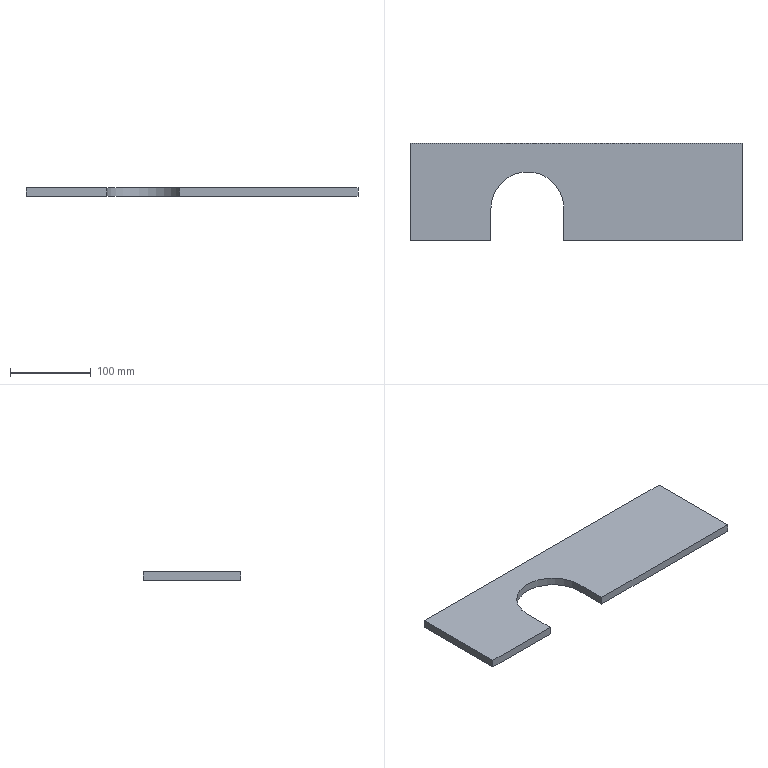Part | NX | features solid 2 | 1 solid | 10 faces | box 410 x 120 x 10 mm | volume 424191 mm3 | plane 9 | cylinder 1 | commonest cylinder face diameters 90 x1
STEP:
#1=CARTESIAN_POINT('',(615.,-830.,-625.));
#2=VERTEX_POINT('',#1);
#3=CARTESIAN_POINT('',(615.,-950.,-625.));
#4=VERTEX_POINT('',#3);
#5=CARTESIAN_POINT('',(615.,-529.496,-625.));
#6=DIRECTION('',(0.,-1.,0.));
#7=VECTOR('',#6,1000.);
#8=LINE('',#5,#7);
#9=EDGE_CURVE('',#2,#4,#8,.T.);
#10=ORIENTED_EDGE('',*,*,#9,.T.);
#11=CARTESIAN_POINT('',(615.,-950.,-635.));
#12=VERTEX_POINT('',#11);
#13=CARTESIAN_POINT('',(615.,-950.,-635.));
#14=DIRECTION('',(0.,0.,1.));
#15=VECTOR('',#14,1000.);
#16=LINE('',#13,#15);
#17=EDGE_CURVE('',#12,#4,#16,.T.);
#18=ORIENTED_EDGE('',*,*,#17,.F.);
#19=CARTESIAN_POINT('',(615.,-830.,-635.));
#20=VERTEX_POINT('',#19);
#21=CARTESIAN_POINT('',(615.,-529.496,-635.));
#22=DIRECTION('',(0.,-1.,0.));
#23=VECTOR('',#22,1000.);
#24=LINE('',#21,#23);
#25=EDGE_CURVE('',#20,#12,#24,.T.);
#26=ORIENTED_EDGE('',*,*,#25,.F.);
#27=CARTESIAN_POINT('',(615.,-830.,-635.));
#28=DIRECTION('',(0.,0.,1.));
#29=VECTOR('',#28,1000.);
#30=LINE('',#27,#29);
#31=EDGE_CURVE('',#20,#2,#30,.T.);
#32=ORIENTED_EDGE('',*,*,#31,.T.);
#33=EDGE_LOOP('',(#10,#18,#26,#32));
#34=FACE_BOUND('',#33,.T.);
#35=CARTESIAN_POINT('',(615.,-529.496,-635.));
#36=DIRECTION('',(-1.,0.,0.));
#37=DIRECTION('',(0.,0.,1.));
#38=AXIS2_PLACEMENT_3D('',#35,#36,#37);
#39=PLANE('',#38);
#40=ADVANCED_FACE('',(#34),#39,.F.);
#41=CARTESIAN_POINT('',(205.,-830.,-625.));
#42=VERTEX_POINT('',#41);
#43=CARTESIAN_POINT('',(-1070.,-830.,-625.));
#44=DIRECTION('',(1.,0.,0.));
#45=VECTOR('',#44,1000.);
#46=LINE('',#43,#45);
#47=EDGE_CURVE('',#42,#2,#46,.T.);
#48=ORIENTED_EDGE('',*,*,#47,.T.);
#49=ORIENTED_EDGE('',*,*,#31,.F.);
#50=CARTESIAN_POINT('',(205.,-830.,-635.));
#51=VERTEX_POINT('',#50);
#52=CARTESIAN_POINT('',(-1070.,-830.,-635.));
#53=DIRECTION('',(1.,0.,0.));
#54=VECTOR('',#53,1000.);
#55=LINE('',#52,#54);
#56=EDGE_CURVE('',#51,#20,#55,.T.);
#57=ORIENTED_EDGE('',*,*,#56,.F.);
#58=CARTESIAN_POINT('',(205.,-830.,-635.));
#59=DIRECTION('',(0.,0.,1.));
#60=VECTOR('',#59,1000.);
#61=LINE('',#58,#60);
#62=EDGE_CURVE('',#51,#42,#61,.T.);
#63=ORIENTED_EDGE('',*,*,#62,.T.);
#64=EDGE_LOOP('',(#48,#49,#57,#63));
#65=FACE_BOUND('',#64,.T.);
#66=CARTESIAN_POINT('',(-1070.,-830.,-635.));
#67=DIRECTION('',(0.,-1.,0.));
#68=DIRECTION('',(1.,0.,0.));
#69=AXIS2_PLACEMENT_3D('',#66,#67,#68);
#70=PLANE('',#69);
#71=ADVANCED_FACE('',(#65),#70,.F.);
#72=CARTESIAN_POINT('',(205.,-950.,-625.));
#73=VERTEX_POINT('',#72);
#74=CARTESIAN_POINT('',(205.,-950.,-625.));
#75=DIRECTION('',(0.,-1.,0.));
#76=VECTOR('',#75,1000.);
#77=LINE('',#74,#76);
#78=EDGE_CURVE('',#42,#73,#77,.T.);
#79=ORIENTED_EDGE('',*,*,#78,.F.);
#80=ORIENTED_EDGE('',*,*,#62,.F.);
#81=CARTESIAN_POINT('',(205.,-950.,-635.));
#82=VERTEX_POINT('',#81);
#83=CARTESIAN_POINT('',(205.,-950.,-635.));
#84=DIRECTION('',(0.,-1.,0.));
#85=VECTOR('',#84,1000.);
#86=LINE('',#83,#85);
#87=EDGE_CURVE('',#51,#82,#86,.T.);
#88=ORIENTED_EDGE('',*,*,#87,.T.);
#89=CARTESIAN_POINT('',(205.,-950.,-635.));
#90=DIRECTION('',(0.,0.,1.));
#91=VECTOR('',#90,1000.);
#92=LINE('',#89,#91);
#93=EDGE_CURVE('',#82,#73,#92,.T.);
#94=ORIENTED_EDGE('',*,*,#93,.T.);
#95=EDGE_LOOP('',(#79,#80,#88,#94));
#96=FACE_BOUND('',#95,.T.);
#97=CARTESIAN_POINT('',(205.,-950.,-635.));
#98=DIRECTION('',(-1.,0.,0.));
#99=DIRECTION('',(0.,0.,1.));
#100=AXIS2_PLACEMENT_3D('',#97,#98,#99);
#101=PLANE('',#100);
#102=ADVANCED_FACE('',(#96),#101,.T.);
#103=CARTESIAN_POINT('',(305.,-950.,-625.));
#104=VERTEX_POINT('',#103);
#105=CARTESIAN_POINT('',(-70.,-950.,-625.));
#106=DIRECTION('',(-1.,0.,0.));
#107=VECTOR('',#106,1000.);
#108=LINE('',#105,#107);
#109=EDGE_CURVE('',#104,#73,#108,.T.);
#110=ORIENTED_EDGE('',*,*,#109,.T.);
#111=ORIENTED_EDGE('',*,*,#93,.F.);
#112=CARTESIAN_POINT('',(305.,-950.,-635.));
#113=VERTEX_POINT('',#112);
#114=CARTESIAN_POINT('',(-70.,-950.,-635.));
#115=DIRECTION('',(-1.,0.,0.));
#116=VECTOR('',#115,1000.);
#117=LINE('',#114,#116);
#118=EDGE_CURVE('',#113,#82,#117,.T.);
#119=ORIENTED_EDGE('',*,*,#118,.F.);
#120=CARTESIAN_POINT('',(305.,-950.,-635.));
#121=DIRECTION('',(0.,0.,1.));
#122=VECTOR('',#121,1000.);
#123=LINE('',#120,#122);
#124=EDGE_CURVE('',#113,#104,#123,.T.);
#125=ORIENTED_EDGE('',*,*,#124,.T.);
#126=EDGE_LOOP('',(#110,#111,#119,#125));
#127=FACE_BOUND('',#126,.T.);
#128=CARTESIAN_POINT('',(-70.,-950.,-635.));
#129=DIRECTION('',(0.,1.,0.));
#130=DIRECTION('',(0.,0.,1.));
#131=AXIS2_PLACEMENT_3D('',#128,#129,#130);
#132=PLANE('',#131);
#133=ADVANCED_FACE('',(#127),#132,.F.);
#134=CARTESIAN_POINT('',(305.,-910.,-625.));
#135=VERTEX_POINT('',#134);
#136=CARTESIAN_POINT('',(305.,-950.,-625.));
#137=DIRECTION('',(0.,1.,0.));
#138=VECTOR('',#137,1000.);
#139=LINE('',#136,#138);
#140=EDGE_CURVE('',#104,#135,#139,.T.);
#141=ORIENTED_EDGE('',*,*,#140,.F.);
#142=ORIENTED_EDGE('',*,*,#124,.F.);
#143=CARTESIAN_POINT('',(305.,-910.,-635.));
#144=VERTEX_POINT('',#143);
#145=CARTESIAN_POINT('',(305.,-950.,-635.));
#146=DIRECTION('',(0.,1.,0.));
#147=VECTOR('',#146,1000.);
#148=LINE('',#145,#147);
#149=EDGE_CURVE('',#113,#144,#148,.T.);
#150=ORIENTED_EDGE('',*,*,#149,.T.);
#151=CARTESIAN_POINT('',(305.,-910.,-635.));
#152=DIRECTION('',(0.,0.,1.));
#153=VECTOR('',#152,1000.);
#154=LINE('',#151,#153);
#155=EDGE_CURVE('',#144,#135,#154,.T.);
#156=ORIENTED_EDGE('',*,*,#155,.T.);
#157=EDGE_LOOP('',(#141,#142,#150,#156));
#158=FACE_BOUND('',#157,.T.);
#159=CARTESIAN_POINT('',(305.,-950.,-635.));
#160=DIRECTION('',(1.,0.,0.));
#161=DIRECTION('',(0.,1.,0.));
#162=AXIS2_PLACEMENT_3D('',#159,#160,#161);
#163=PLANE('',#162);
#164=ADVANCED_FACE('',(#158),#163,.T.);
#165=CARTESIAN_POINT('',(395.,-910.,-625.));
#166=VERTEX_POINT('',#165);
#167=CARTESIAN_POINT('',(350.,-910.,-625.));
#168=DIRECTION('',(0.,0.,1.));
#169=DIRECTION('',(1.,0.,0.));
#170=AXIS2_PLACEMENT_3D('',#167,#168,#169);
#171=CIRCLE('',#170,45.);
#172=EDGE_CURVE('',#166,#135,#171,.T.);
#173=ORIENTED_EDGE('',*,*,#172,.T.);
#174=ORIENTED_EDGE('',*,*,#155,.F.);
#175=CARTESIAN_POINT('',(395.,-910.,-635.));
#176=VERTEX_POINT('',#175);
#177=CARTESIAN_POINT('',(350.,-910.,-635.));
#178=DIRECTION('',(0.,0.,1.));
#179=DIRECTION('',(1.,0.,0.));
#180=AXIS2_PLACEMENT_3D('',#177,#178,#179);
#181=CIRCLE('',#180,45.);
#182=EDGE_CURVE('',#176,#144,#181,.T.);
#183=ORIENTED_EDGE('',*,*,#182,.F.);
#184=CARTESIAN_POINT('',(395.,-910.,-635.));
#185=DIRECTION('',(0.,0.,1.));
#186=VECTOR('',#185,1000.);
#187=LINE('',#184,#186);
#188=EDGE_CURVE('',#176,#166,#187,.T.);
#189=ORIENTED_EDGE('',*,*,#188,.T.);
#190=EDGE_LOOP('',(#173,#174,#183,#189));
#191=FACE_BOUND('',#190,.T.);
#192=CARTESIAN_POINT('',(350.,-910.,-635.));
#193=DIRECTION('',(0.,0.,1.));
#194=DIRECTION('',(1.,0.,0.));
#195=AXIS2_PLACEMENT_3D('',#192,#193,#194);
#196=CYLINDRICAL_SURFACE('',#195,45.);
#197=ADVANCED_FACE('',(#191),#196,.F.);
#198=CARTESIAN_POINT('',(395.,-950.,-625.));
#199=VERTEX_POINT('',#198);
#200=CARTESIAN_POINT('',(395.,-910.,-625.));
#201=DIRECTION('',(0.,-1.,0.));
#202=VECTOR('',#201,1000.);
#203=LINE('',#200,#202);
#204=EDGE_CURVE('',#166,#199,#203,.T.);
#205=ORIENTED_EDGE('',*,*,#204,.F.);
#206=ORIENTED_EDGE('',*,*,#188,.F.);
#207=CARTESIAN_POINT('',(395.,-950.,-635.));
#208=VERTEX_POINT('',#207);
#209=CARTESIAN_POINT('',(395.,-910.,-635.));
#210=DIRECTION('',(0.,-1.,0.));
#211=VECTOR('',#210,1000.);
#212=LINE('',#209,#211);
#213=EDGE_CURVE('',#176,#208,#212,.T.);
#214=ORIENTED_EDGE('',*,*,#213,.T.);
#215=CARTESIAN_POINT('',(395.,-950.,-635.));
#216=DIRECTION('',(0.,0.,1.));
#217=VECTOR('',#216,1000.);
#218=LINE('',#215,#217);
#219=EDGE_CURVE('',#208,#199,#218,.T.);
#220=ORIENTED_EDGE('',*,*,#219,.T.);
#221=EDGE_LOOP('',(#205,#206,#214,#220));
#222=FACE_BOUND('',#221,.T.);
#223=CARTESIAN_POINT('',(395.,-910.,-635.));
#224=DIRECTION('',(-1.,0.,0.));
#225=DIRECTION('',(0.,-1.,0.));
#226=AXIS2_PLACEMENT_3D('',#223,#224,#225);
#227=PLANE('',#226);
#228=ADVANCED_FACE('',(#222),#227,.T.);
#229=CARTESIAN_POINT('',(780.,-950.,-625.));
#230=DIRECTION('',(-1.,0.,0.));
#231=VECTOR('',#230,1000.);
#232=LINE('',#229,#231);
#233=EDGE_CURVE('',#4,#199,#232,.T.);
#234=ORIENTED_EDGE('',*,*,#233,.T.);
#235=ORIENTED_EDGE('',*,*,#219,.F.);
#236=CARTESIAN_POINT('',(780.,-950.,-635.));
#237=DIRECTION('',(-1.,0.,0.));
#238=VECTOR('',#237,1000.);
#239=LINE('',#236,#238);
#240=EDGE_CURVE('',#12,#208,#239,.T.);
#241=ORIENTED_EDGE('',*,*,#240,.F.);
#242=ORIENTED_EDGE('',*,*,#17,.T.);
#243=EDGE_LOOP('',(#234,#235,#241,#242));
#244=FACE_BOUND('',#243,.T.);
#245=CARTESIAN_POINT('',(780.,-950.,-635.));
#246=DIRECTION('',(0.,1.,0.));
#247=DIRECTION('',(-1.,0.,0.));
#248=AXIS2_PLACEMENT_3D('',#245,#246,#247);
#249=PLANE('',#248);
#250=ADVANCED_FACE('',(#244),#249,.F.);
#251=ORIENTED_EDGE('',*,*,#25,.T.);
#252=ORIENTED_EDGE('',*,*,#240,.T.);
#253=ORIENTED_EDGE('',*,*,#213,.F.);
#254=ORIENTED_EDGE('',*,*,#182,.T.);
#255=ORIENTED_EDGE('',*,*,#149,.F.);
#256=ORIENTED_EDGE('',*,*,#118,.T.);
#257=ORIENTED_EDGE('',*,*,#87,.F.);
#258=ORIENTED_EDGE('',*,*,#56,.T.);
#259=EDGE_LOOP('',(#251,#252,#253,#254,#255,#256,#257,#258));
#260=FACE_BOUND('',#259,.T.);
#261=CARTESIAN_POINT('',(780.,-950.,-635.));
#262=DIRECTION('',(0.,0.,-1.));
#263=DIRECTION('',(-1.,0.,0.));
#264=AXIS2_PLACEMENT_3D('',#261,#262,#263);
#265=PLANE('',#264);
#266=ADVANCED_FACE('',(#260),#265,.T.);
#267=ORIENTED_EDGE('',*,*,#9,.F.);
#268=ORIENTED_EDGE('',*,*,#47,.F.);
#269=ORIENTED_EDGE('',*,*,#78,.T.);
#270=ORIENTED_EDGE('',*,*,#109,.F.);
#271=ORIENTED_EDGE('',*,*,#140,.T.);
#272=ORIENTED_EDGE('',*,*,#172,.F.);
#273=ORIENTED_EDGE('',*,*,#204,.T.);
#274=ORIENTED_EDGE('',*,*,#233,.F.);
#275=EDGE_LOOP('',(#267,#268,#269,#270,#271,#272,#273,#274));
#276=FACE_BOUND('',#275,.T.);
#277=CARTESIAN_POINT('',(780.,-950.,-625.));
#278=DIRECTION('',(0.,0.,-1.));
#279=DIRECTION('',(-1.,0.,0.));
#280=AXIS2_PLACEMENT_3D('',#277,#278,#279);
#281=PLANE('',#280);
#282=ADVANCED_FACE('',(#276),#281,.F.);
#283=CLOSED_SHELL('',(#40,#71,#102,#133,#164,#197,#228,#250,#266,#282));
#284=MANIFOLD_SOLID_BREP('',#283);
#285=(LENGTH_UNIT()NAMED_UNIT(*)SI_UNIT(.MILLI.,.METRE.));
#286=UNCERTAINTY_MEASURE_WITH_UNIT(LENGTH_MEASURE(0.00001),#285,'','');
#287=(NAMED_UNIT(*)PLANE_ANGLE_UNIT()SI_UNIT($,.RADIAN.));
#288=(NAMED_UNIT(*)SI_UNIT($,.STERADIAN.)SOLID_ANGLE_UNIT());
#289=(GEOMETRIC_REPRESENTATION_CONTEXT(3)GLOBAL_UNCERTAINTY_ASSIGNED_CONTEXT((#286))GLOBAL_UNIT_ASSIGNED_CONTEXT((#285,#287,#288))REPRESENTATION_CONTEXT('',''));
#290=ADVANCED_BREP_SHAPE_REPRESENTATION('',(#284),#289);